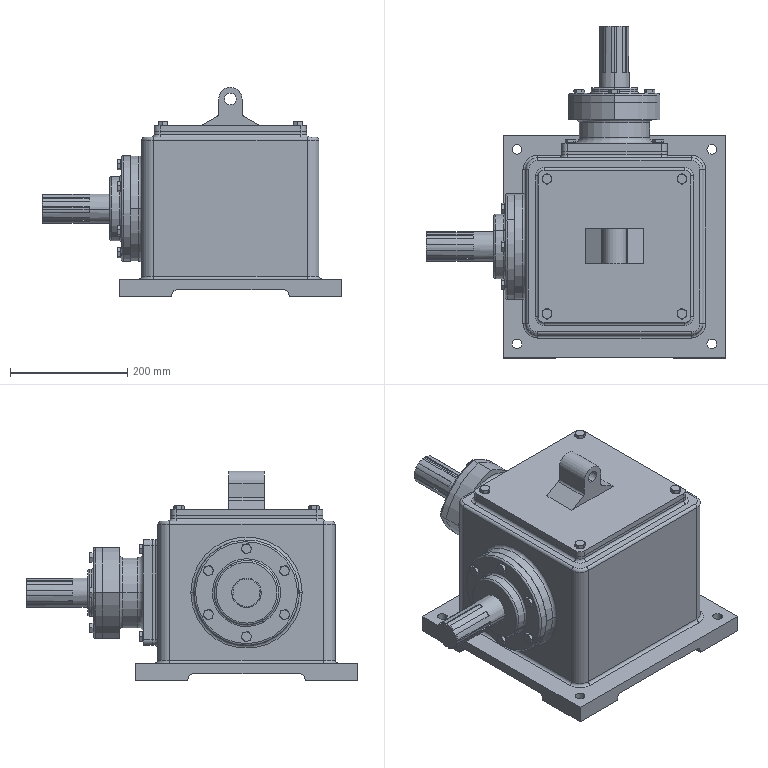Part | SolidWorks | features ReferencePattern 5, CompositeCurve 3, LocalCirPattern 1 | 37 solids | 2064 faces | box 510.982 x 565.982 x 357 mm | volume 19755634 mm3 | plane 561 | cylinder 471 | cone 362 | sphere 320 | torus 248 | spline 102 | commonest cylinder face diameters 10 x54 8.5 x36 10.5 x36 16 x36 81 x32 20 x26